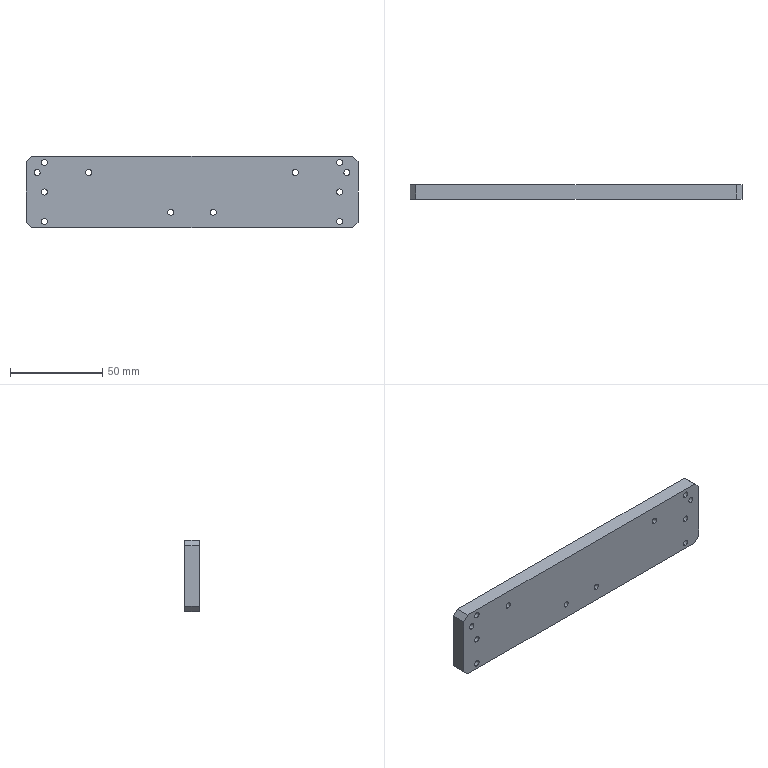Part | STEP file | 0-10-28 Cylinder mounting plate | 1 solid | 34 faces | box 180 x 8 x 39 mm | volume 55195 mm3 | cylinder 24 | plane 10 | commonest cylinder face diameters 3.3 x24